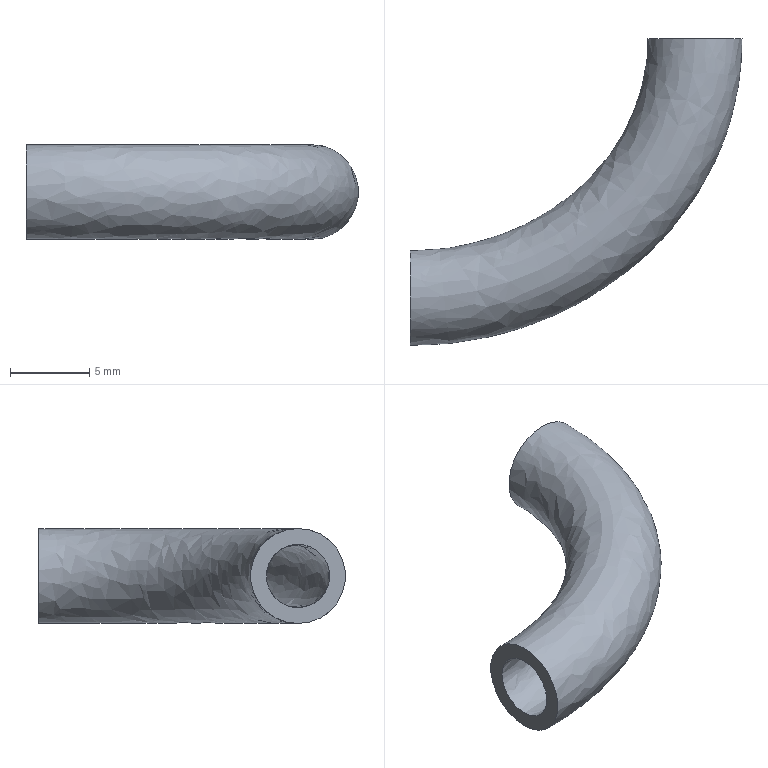Part | NX | features solid 2 | 1 solid | 4 faces | box 21 x 19.402 x 6 mm | volume 425.824 mm3 | plane 2 | spline 2